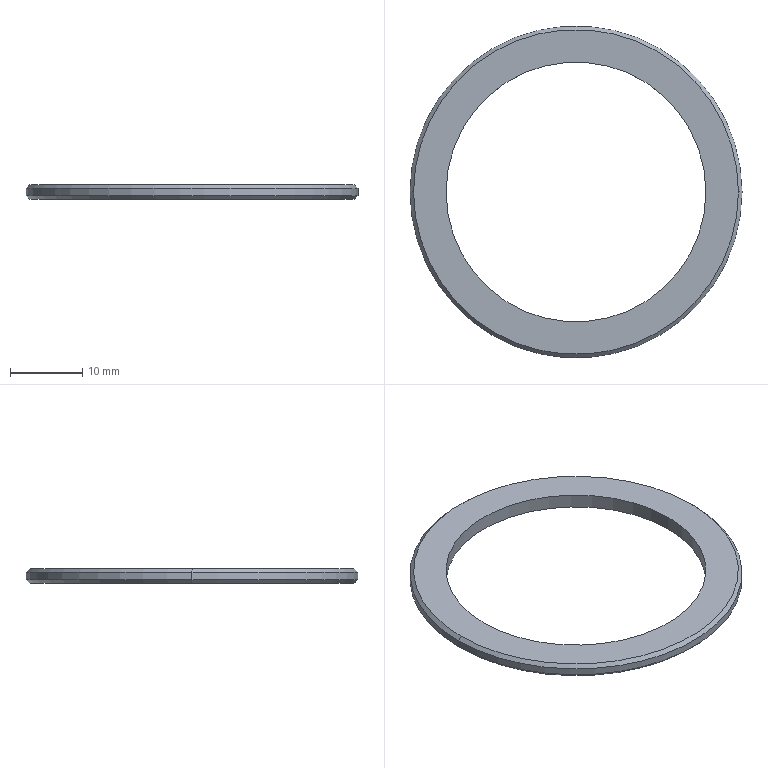Part | STEP file | HXGR200008-06-02-01 | 1 solid | 10 faces | box 46 x 46 x 2 mm | volume 1252 mm3 | cone 4 | cylinder 4 | plane 2 | commonest cylinder face diameters 36 x2 46 x2
STEP:
#1=CARTESIAN_POINT('',(22.5,0.,0.));
#2=VERTEX_POINT('',#1);
#3=CARTESIAN_POINT('',(-22.5,0.,0.));
#4=VERTEX_POINT('',#3);
#5=CARTESIAN_POINT('',(0.,0.,0.));
#6=DIRECTION('',(0.,0.,1.));
#7=DIRECTION('',(1.,0.,0.));
#8=AXIS2_PLACEMENT_3D('',#5,#6,#7);
#9=CIRCLE('',#8,22.5);
#10=EDGE_CURVE('',#2,#4,#9,.T.);
#11=ORIENTED_EDGE('',*,*,#10,.F.);
#12=CARTESIAN_POINT('',(23.,0.,-0.5));
#13=VERTEX_POINT('',#12);
#14=CARTESIAN_POINT('',(22.5,0.,0.));
#15=DIRECTION('',(0.7071,0.,-0.7071));
#16=VECTOR('',#15,1000.);
#17=LINE('',#14,#16);
#18=EDGE_CURVE('',#2,#13,#17,.T.);
#19=ORIENTED_EDGE('',*,*,#18,.T.);
#20=CARTESIAN_POINT('',(-23.,0.,-0.5));
#21=VERTEX_POINT('',#20);
#22=CARTESIAN_POINT('',(0.,0.,-0.5));
#23=DIRECTION('',(0.,0.,-1.));
#24=DIRECTION('',(1.,0.,0.));
#25=AXIS2_PLACEMENT_3D('',#22,#23,#24);
#26=CIRCLE('',#25,23.);
#27=EDGE_CURVE('',#21,#13,#26,.T.);
#28=ORIENTED_EDGE('',*,*,#27,.F.);
#29=CARTESIAN_POINT('',(-22.5,0.,0.));
#30=DIRECTION('',(-0.7071,0.,-0.7071));
#31=VECTOR('',#30,1000.);
#32=LINE('',#29,#31);
#33=EDGE_CURVE('',#4,#21,#32,.T.);
#34=ORIENTED_EDGE('',*,*,#33,.F.);
#35=EDGE_LOOP('',(#11,#19,#28,#34));
#36=FACE_OUTER_BOUND('',#35,.T.);
#37=CARTESIAN_POINT('',(0.,0.,0.));
#38=DIRECTION('',(0.,0.,-1.));
#39=DIRECTION('',(-1.,0.,0.));
#40=AXIS2_PLACEMENT_3D('',#37,#38,#39);
#41=CONICAL_SURFACE('',#40,22.5,0.7854);
#42=ADVANCED_FACE('',(#36),#41,.T.);
#43=CARTESIAN_POINT('',(-22.5,0.,-2.));
#44=VERTEX_POINT('',#43);
#45=CARTESIAN_POINT('',(22.5,0.,-2.));
#46=VERTEX_POINT('',#45);
#47=CARTESIAN_POINT('',(0.,0.,-2.));
#48=DIRECTION('',(0.,0.,-1.));
#49=DIRECTION('',(1.,0.,0.));
#50=AXIS2_PLACEMENT_3D('',#47,#48,#49);
#51=CIRCLE('',#50,22.5);
#52=EDGE_CURVE('',#44,#46,#51,.T.);
#53=ORIENTED_EDGE('',*,*,#52,.F.);
#54=CARTESIAN_POINT('',(-23.,0.,-1.5));
#55=VERTEX_POINT('',#54);
#56=CARTESIAN_POINT('',(-23.,0.,-1.5));
#57=DIRECTION('',(-0.7071,0.,0.7071));
#58=VECTOR('',#57,1000.);
#59=LINE('',#56,#58);
#60=EDGE_CURVE('',#44,#55,#59,.T.);
#61=ORIENTED_EDGE('',*,*,#60,.T.);
#62=CARTESIAN_POINT('',(23.,0.,-1.5));
#63=VERTEX_POINT('',#62);
#64=CARTESIAN_POINT('',(0.,0.,-1.5));
#65=DIRECTION('',(0.,0.,1.));
#66=DIRECTION('',(1.,0.,0.));
#67=AXIS2_PLACEMENT_3D('',#64,#65,#66);
#68=CIRCLE('',#67,23.);
#69=EDGE_CURVE('',#63,#55,#68,.T.);
#70=ORIENTED_EDGE('',*,*,#69,.F.);
#71=CARTESIAN_POINT('',(23.,0.,-1.5));
#72=DIRECTION('',(0.7071,0.,0.7071));
#73=VECTOR('',#72,1000.);
#74=LINE('',#71,#73);
#75=EDGE_CURVE('',#46,#63,#74,.T.);
#76=ORIENTED_EDGE('',*,*,#75,.F.);
#77=EDGE_LOOP('',(#53,#61,#70,#76));
#78=FACE_OUTER_BOUND('',#77,.T.);
#79=CARTESIAN_POINT('',(0.,0.,-1.5));
#80=DIRECTION('',(0.,0.,1.));
#81=DIRECTION('',(1.,0.,0.));
#82=AXIS2_PLACEMENT_3D('',#79,#80,#81);
#83=CONICAL_SURFACE('',#82,23.,0.7854);
#84=ADVANCED_FACE('',(#78),#83,.T.);
#85=CARTESIAN_POINT('',(-18.,0.,-2.));
#86=VERTEX_POINT('',#85);
#87=CARTESIAN_POINT('',(18.,0.,-2.));
#88=VERTEX_POINT('',#87);
#89=CARTESIAN_POINT('',(0.,0.,-2.));
#90=DIRECTION('',(0.,0.,1.));
#91=DIRECTION('',(1.,0.,0.));
#92=AXIS2_PLACEMENT_3D('',#89,#90,#91);
#93=CIRCLE('',#92,18.);
#94=EDGE_CURVE('',#86,#88,#93,.T.);
#95=ORIENTED_EDGE('',*,*,#94,.F.);
#96=CARTESIAN_POINT('',(-18.,0.,0.));
#97=VERTEX_POINT('',#96);
#98=CARTESIAN_POINT('',(-18.,0.,-2.));
#99=DIRECTION('',(0.,0.,1.));
#100=VECTOR('',#99,1000.);
#101=LINE('',#98,#100);
#102=EDGE_CURVE('',#86,#97,#101,.T.);
#103=ORIENTED_EDGE('',*,*,#102,.T.);
#104=CARTESIAN_POINT('',(18.,0.,0.));
#105=VERTEX_POINT('',#104);
#106=CARTESIAN_POINT('',(0.,0.,0.));
#107=DIRECTION('',(0.,0.,1.));
#108=DIRECTION('',(1.,0.,0.));
#109=AXIS2_PLACEMENT_3D('',#106,#107,#108);
#110=CIRCLE('',#109,18.);
#111=EDGE_CURVE('',#97,#105,#110,.T.);
#112=ORIENTED_EDGE('',*,*,#111,.T.);
#113=CARTESIAN_POINT('',(18.,0.,-2.));
#114=DIRECTION('',(0.,0.,1.));
#115=VECTOR('',#114,1000.);
#116=LINE('',#113,#115);
#117=EDGE_CURVE('',#88,#105,#116,.T.);
#118=ORIENTED_EDGE('',*,*,#117,.F.);
#119=EDGE_LOOP('',(#95,#103,#112,#118));
#120=FACE_OUTER_BOUND('',#119,.T.);
#121=CARTESIAN_POINT('',(0.,0.,-2.));
#122=DIRECTION('',(0.,0.,1.));
#123=DIRECTION('',(1.,0.,0.));
#124=AXIS2_PLACEMENT_3D('',#121,#122,#123);
#125=CYLINDRICAL_SURFACE('',#124,18.);
#126=ADVANCED_FACE('',(#120),#125,.F.);
#127=ORIENTED_EDGE('',*,*,#69,.T.);
#128=CARTESIAN_POINT('',(-23.,0.,-2.));
#129=DIRECTION('',(0.,0.,1.));
#130=VECTOR('',#129,1000.);
#131=LINE('',#128,#130);
#132=EDGE_CURVE('',#55,#21,#131,.T.);
#133=ORIENTED_EDGE('',*,*,#132,.T.);
#134=ORIENTED_EDGE('',*,*,#27,.T.);
#135=CARTESIAN_POINT('',(23.,0.,-2.));
#136=DIRECTION('',(0.,0.,1.));
#137=VECTOR('',#136,1000.);
#138=LINE('',#135,#137);
#139=EDGE_CURVE('',#63,#13,#138,.T.);
#140=ORIENTED_EDGE('',*,*,#139,.F.);
#141=EDGE_LOOP('',(#127,#133,#134,#140));
#142=FACE_OUTER_BOUND('',#141,.T.);
#143=CARTESIAN_POINT('',(0.,0.,-2.));
#144=DIRECTION('',(0.,0.,1.));
#145=DIRECTION('',(1.,0.,0.));
#146=AXIS2_PLACEMENT_3D('',#143,#144,#145);
#147=CYLINDRICAL_SURFACE('',#146,23.);
#148=ADVANCED_FACE('',(#142),#147,.T.);
#149=ORIENTED_EDGE('',*,*,#132,.F.);
#150=CARTESIAN_POINT('',(0.,0.,-1.5));
#151=DIRECTION('',(0.,0.,1.));
#152=DIRECTION('',(1.,0.,0.));
#153=AXIS2_PLACEMENT_3D('',#150,#151,#152);
#154=CIRCLE('',#153,23.);
#155=EDGE_CURVE('',#55,#63,#154,.T.);
#156=ORIENTED_EDGE('',*,*,#155,.T.);
#157=ORIENTED_EDGE('',*,*,#139,.T.);
#158=CARTESIAN_POINT('',(0.,0.,-0.5));
#159=DIRECTION('',(0.,0.,-1.));
#160=DIRECTION('',(1.,0.,0.));
#161=AXIS2_PLACEMENT_3D('',#158,#159,#160);
#162=CIRCLE('',#161,23.);
#163=EDGE_CURVE('',#13,#21,#162,.T.);
#164=ORIENTED_EDGE('',*,*,#163,.T.);
#165=EDGE_LOOP('',(#149,#156,#157,#164));
#166=FACE_OUTER_BOUND('',#165,.T.);
#167=CARTESIAN_POINT('',(0.,0.,-2.));
#168=DIRECTION('',(0.,0.,1.));
#169=DIRECTION('',(1.,0.,0.));
#170=AXIS2_PLACEMENT_3D('',#167,#168,#169);
#171=CYLINDRICAL_SURFACE('',#170,23.);
#172=ADVANCED_FACE('',(#166),#171,.T.);
#173=CARTESIAN_POINT('',(0.,0.,-2.));
#174=DIRECTION('',(0.,0.,-1.));
#175=DIRECTION('',(1.,0.,0.));
#176=AXIS2_PLACEMENT_3D('',#173,#174,#175);
#177=CIRCLE('',#176,22.5);
#178=EDGE_CURVE('',#46,#44,#177,.T.);
#179=ORIENTED_EDGE('',*,*,#178,.T.);
#180=ORIENTED_EDGE('',*,*,#52,.T.);
#181=EDGE_LOOP('',(#179,#180));
#182=FACE_OUTER_BOUND('',#181,.T.);
#183=CARTESIAN_POINT('',(0.,0.,-2.));
#184=DIRECTION('',(0.,0.,1.));
#185=DIRECTION('',(1.,0.,0.));
#186=AXIS2_PLACEMENT_3D('',#183,#184,#185);
#187=CIRCLE('',#186,18.);
#188=EDGE_CURVE('',#88,#86,#187,.T.);
#189=ORIENTED_EDGE('',*,*,#188,.T.);
#190=ORIENTED_EDGE('',*,*,#94,.T.);
#191=EDGE_LOOP('',(#189,#190));
#192=FACE_BOUND('',#191,.T.);
#193=CARTESIAN_POINT('',(0.,0.,-2.));
#194=DIRECTION('',(0.,0.,1.));
#195=DIRECTION('',(1.,0.,0.));
#196=AXIS2_PLACEMENT_3D('',#193,#194,#195);
#197=PLANE('',#196);
#198=ADVANCED_FACE('',(#182,#192),#197,.F.);
#199=CARTESIAN_POINT('',(0.,0.,0.));
#200=DIRECTION('',(0.,0.,1.));
#201=DIRECTION('',(1.,0.,0.));
#202=AXIS2_PLACEMENT_3D('',#199,#200,#201);
#203=CIRCLE('',#202,22.5);
#204=EDGE_CURVE('',#4,#2,#203,.T.);
#205=ORIENTED_EDGE('',*,*,#204,.T.);
#206=ORIENTED_EDGE('',*,*,#10,.T.);
#207=EDGE_LOOP('',(#205,#206));
#208=FACE_OUTER_BOUND('',#207,.T.);
#209=CARTESIAN_POINT('',(0.,0.,0.));
#210=DIRECTION('',(0.,0.,1.));
#211=DIRECTION('',(1.,0.,0.));
#212=AXIS2_PLACEMENT_3D('',#209,#210,#211);
#213=CIRCLE('',#212,18.);
#214=EDGE_CURVE('',#105,#97,#213,.T.);
#215=ORIENTED_EDGE('',*,*,#214,.F.);
#216=ORIENTED_EDGE('',*,*,#111,.F.);
#217=EDGE_LOOP('',(#215,#216));
#218=FACE_BOUND('',#217,.T.);
#219=CARTESIAN_POINT('',(0.,0.,0.));
#220=DIRECTION('',(0.,0.,1.));
#221=DIRECTION('',(1.,0.,0.));
#222=AXIS2_PLACEMENT_3D('',#219,#220,#221);
#223=PLANE('',#222);
#224=ADVANCED_FACE('',(#208,#218),#223,.T.);
#225=ORIENTED_EDGE('',*,*,#102,.F.);
#226=ORIENTED_EDGE('',*,*,#188,.F.);
#227=ORIENTED_EDGE('',*,*,#117,.T.);
#228=ORIENTED_EDGE('',*,*,#214,.T.);
#229=EDGE_LOOP('',(#225,#226,#227,#228));
#230=FACE_OUTER_BOUND('',#229,.T.);
#231=CARTESIAN_POINT('',(0.,0.,-2.));
#232=DIRECTION('',(0.,0.,1.));
#233=DIRECTION('',(1.,0.,0.));
#234=AXIS2_PLACEMENT_3D('',#231,#232,#233);
#235=CYLINDRICAL_SURFACE('',#234,18.);
#236=ADVANCED_FACE('',(#230),#235,.F.);
#237=ORIENTED_EDGE('',*,*,#60,.F.);
#238=ORIENTED_EDGE('',*,*,#178,.F.);
#239=ORIENTED_EDGE('',*,*,#75,.T.);
#240=ORIENTED_EDGE('',*,*,#155,.F.);
#241=EDGE_LOOP('',(#237,#238,#239,#240));
#242=FACE_OUTER_BOUND('',#241,.T.);
#243=CARTESIAN_POINT('',(0.,0.,-1.5));
#244=DIRECTION('',(0.,0.,1.));
#245=DIRECTION('',(1.,0.,0.));
#246=AXIS2_PLACEMENT_3D('',#243,#244,#245);
#247=CONICAL_SURFACE('',#246,23.,0.7854);
#248=ADVANCED_FACE('',(#242),#247,.T.);
#249=ORIENTED_EDGE('',*,*,#18,.F.);
#250=ORIENTED_EDGE('',*,*,#204,.F.);
#251=ORIENTED_EDGE('',*,*,#33,.T.);
#252=ORIENTED_EDGE('',*,*,#163,.F.);
#253=EDGE_LOOP('',(#249,#250,#251,#252));
#254=FACE_OUTER_BOUND('',#253,.T.);
#255=CARTESIAN_POINT('',(0.,0.,0.));
#256=DIRECTION('',(0.,0.,-1.));
#257=DIRECTION('',(-1.,0.,0.));
#258=AXIS2_PLACEMENT_3D('',#255,#256,#257);
#259=CONICAL_SURFACE('',#258,22.5,0.7854);
#260=ADVANCED_FACE('',(#254),#259,.T.);
#261=CLOSED_SHELL('',(#42,#84,#126,#148,#172,#198,#224,#236,#248,#260));
#262=MANIFOLD_SOLID_BREP('',#261);
#263=CARTESIAN_POINT('',(0.,0.,0.));
#264=DIRECTION('',(0.,0.,1.));
#265=DIRECTION('',(1.,0.,0.));
#266=AXIS2_PLACEMENT_3D('',#263,#264,#265);
#267=(LENGTH_UNIT()NAMED_UNIT(*)SI_UNIT(.MILLI.,.METRE.));
#268=UNCERTAINTY_MEASURE_WITH_UNIT(LENGTH_MEASURE(0.00001),#267,'','');
#269=(NAMED_UNIT(*)PLANE_ANGLE_UNIT()SI_UNIT($,.RADIAN.));
#270=(NAMED_UNIT(*)SI_UNIT($,.STERADIAN.)SOLID_ANGLE_UNIT());
#271=(GEOMETRIC_REPRESENTATION_CONTEXT(3)GLOBAL_UNCERTAINTY_ASSIGNED_CONTEXT((#268))GLOBAL_UNIT_ASSIGNED_CONTEXT((#267,#269,#270))REPRESENTATION_CONTEXT('',''));
#272=ADVANCED_BREP_SHAPE_REPRESENTATION('',(#262,#266),#271);